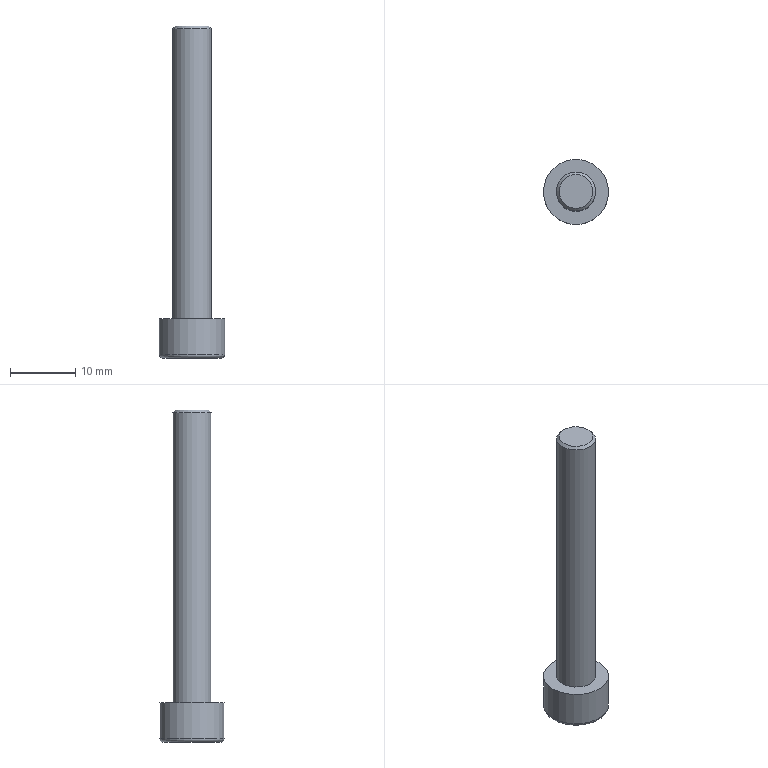Part | STEP file | 200 mesh_id134_x | 1 solid | 20 faces | box 10 x 10 x 51 mm | volume 1654 mm3 | plane 10 | cylinder 8 | torus 1 | cone 1 | commonest cylinder face diameters 0.4 x6 6 x1 10 x1
STEP:
#1=CARTESIAN_POINT('',(-16734.384,-3900.387,88.258));
#2=VERTEX_POINT('',#1);
#3=CARTESIAN_POINT('',(-16731.684,-3898.828,88.258));
#4=VERTEX_POINT('',#3);
#5=CARTESIAN_POINT('',(-16731.784,-3898.886,88.258));
#6=DIRECTION('',(0.866,0.5,0.));
#7=VECTOR('',#6,1.);
#8=LINE('',#5,#7);
#9=EDGE_CURVE('',#2,#4,#8,.T.);
#10=ORIENTED_EDGE('',*,*,#9,.T.);
#11=CARTESIAN_POINT('',(-16731.684,-3895.71,88.258));
#12=VERTEX_POINT('',#11);
#13=CARTESIAN_POINT('',(-16731.684,-3895.826,88.258));
#14=DIRECTION('',(0.,1.,0.));
#15=VECTOR('',#14,1.);
#16=LINE('',#13,#15);
#17=EDGE_CURVE('',#4,#12,#16,.T.);
#18=ORIENTED_EDGE('',*,*,#17,.T.);
#19=CARTESIAN_POINT('',(-16734.384,-3894.151,88.258));
#20=VERTEX_POINT('',#19);
#21=CARTESIAN_POINT('',(-16734.284,-3894.209,88.258));
#22=DIRECTION('',(-0.866,0.5,0.));
#23=VECTOR('',#22,1.);
#24=LINE('',#21,#23);
#25=EDGE_CURVE('',#12,#20,#24,.T.);
#26=ORIENTED_EDGE('',*,*,#25,.T.);
#27=CARTESIAN_POINT('',(-16737.084,-3895.71,88.258));
#28=VERTEX_POINT('',#27);
#29=CARTESIAN_POINT('',(-16736.984,-3895.653,88.258));
#30=DIRECTION('',(-0.866,-0.5,0.));
#31=VECTOR('',#30,1.);
#32=LINE('',#29,#31);
#33=EDGE_CURVE('',#20,#28,#32,.T.);
#34=ORIENTED_EDGE('',*,*,#33,.T.);
#35=CARTESIAN_POINT('',(-16737.084,-3898.828,88.258));
#36=VERTEX_POINT('',#35);
#37=CARTESIAN_POINT('',(-16737.084,-3898.713,88.258));
#38=DIRECTION('',(0.,-1.,0.));
#39=VECTOR('',#38,1.);
#40=LINE('',#37,#39);
#41=EDGE_CURVE('',#28,#36,#40,.T.);
#42=ORIENTED_EDGE('',*,*,#41,.T.);
#43=CARTESIAN_POINT('',(-16734.484,-3900.329,88.258));
#44=DIRECTION('',(0.866,-0.5,0.));
#45=VECTOR('',#44,1.);
#46=LINE('',#43,#45);
#47=EDGE_CURVE('',#36,#2,#46,.T.);
#48=ORIENTED_EDGE('',*,*,#47,.T.);
#49=EDGE_LOOP('',(#10,#18,#26,#34,#42,#48));
#50=FACE_BOUND('',#49,.T.);
#51=CARTESIAN_POINT('',(-16738.884,-3897.269,88.258));
#52=VERTEX_POINT('',#51);
#53=CARTESIAN_POINT('',(-16734.384,-3897.269,88.258));
#54=DIRECTION('',(0.,0.,-1.));
#55=DIRECTION('',(-1.,0.,0.));
#56=AXIS2_PLACEMENT_3D('',#53,#54,#55);
#57=CIRCLE('',#56,4.5);
#58=EDGE_CURVE('',#52,#52,#57,.T.);
#59=ORIENTED_EDGE('',*,*,#58,.T.);
#60=EDGE_LOOP('',(#59));
#61=FACE_BOUND('',#60,.T.);
#62=CARTESIAN_POINT('',(-16734.384,-3897.269,88.258));
#63=DIRECTION('',(0.,0.,-1.));
#64=DIRECTION('',(-1.,0.,0.));
#65=AXIS2_PLACEMENT_3D('',#62,#63,#64);
#66=PLANE('',#65);
#67=ADVANCED_FACE('',(#50,#61),#66,.T.);
#68=CARTESIAN_POINT('',(-16731.384,-3897.269,138.858));
#69=VERTEX_POINT('',#68);
#70=CARTESIAN_POINT('',(-16734.384,-3897.269,138.858));
#71=DIRECTION('',(0.,0.,-1.));
#72=DIRECTION('',(1.,0.,0.));
#73=AXIS2_PLACEMENT_3D('',#70,#71,#72);
#74=CIRCLE('',#73,3.);
#75=EDGE_CURVE('',#69,#69,#74,.T.);
#76=ORIENTED_EDGE('',*,*,#75,.T.);
#77=EDGE_LOOP('',(#76));
#78=FACE_BOUND('',#77,.T.);
#79=CARTESIAN_POINT('',(-16731.384,-3897.269,94.258));
#80=VERTEX_POINT('',#79);
#81=CARTESIAN_POINT('',(-16734.384,-3897.269,94.258));
#82=DIRECTION('',(0.,0.,-1.));
#83=DIRECTION('',(1.,0.,0.));
#84=AXIS2_PLACEMENT_3D('',#81,#82,#83);
#85=CIRCLE('',#84,3.);
#86=EDGE_CURVE('',#80,#80,#85,.T.);
#87=ORIENTED_EDGE('',*,*,#86,.F.);
#88=EDGE_LOOP('',(#87));
#89=FACE_BOUND('',#88,.T.);
#90=CARTESIAN_POINT('',(-16734.384,-3897.269,94.258));
#91=DIRECTION('',(0.,0.,1.));
#92=DIRECTION('',(1.,0.,0.));
#93=AXIS2_PLACEMENT_3D('',#90,#91,#92);
#94=CYLINDRICAL_SURFACE('',#93,3.);
#95=ADVANCED_FACE('',(#78,#89),#94,.T.);
#96=ORIENTED_EDGE('',*,*,#86,.T.);
#97=EDGE_LOOP('',(#96));
#98=FACE_BOUND('',#97,.T.);
#99=CARTESIAN_POINT('',(-16729.384,-3897.269,94.258));
#100=VERTEX_POINT('',#99);
#101=CARTESIAN_POINT('',(-16734.384,-3897.269,94.258));
#102=DIRECTION('',(0.,0.,-1.));
#103=DIRECTION('',(1.,0.,0.));
#104=AXIS2_PLACEMENT_3D('',#101,#102,#103);
#105=CIRCLE('',#104,5.);
#106=EDGE_CURVE('',#100,#100,#105,.T.);
#107=ORIENTED_EDGE('',*,*,#106,.F.);
#108=EDGE_LOOP('',(#107));
#109=FACE_BOUND('',#108,.T.);
#110=CARTESIAN_POINT('',(-16734.384,-3897.269,94.258));
#111=DIRECTION('',(0.,0.,1.));
#112=DIRECTION('',(1.,0.,0.));
#113=AXIS2_PLACEMENT_3D('',#110,#111,#112);
#114=PLANE('',#113);
#115=ADVANCED_FACE('',(#98,#109),#114,.T.);
#116=CARTESIAN_POINT('',(-16739.384,-3897.269,88.758));
#117=VERTEX_POINT('',#116);
#118=CARTESIAN_POINT('',(-16734.384,-3897.269,88.758));
#119=DIRECTION('',(0.,0.,1.));
#120=DIRECTION('',(-1.,0.,0.));
#121=AXIS2_PLACEMENT_3D('',#118,#119,#120);
#122=CIRCLE('',#121,5.);
#123=EDGE_CURVE('',#117,#117,#122,.T.);
#124=ORIENTED_EDGE('',*,*,#123,.T.);
#125=EDGE_LOOP('',(#124));
#126=FACE_BOUND('',#125,.T.);
#127=ORIENTED_EDGE('',*,*,#106,.T.);
#128=EDGE_LOOP('',(#127));
#129=FACE_BOUND('',#128,.T.);
#130=CARTESIAN_POINT('',(-16734.384,-3897.269,94.258));
#131=DIRECTION('',(0.,0.,-1.));
#132=DIRECTION('',(1.,0.,0.));
#133=AXIS2_PLACEMENT_3D('',#130,#131,#132);
#134=CYLINDRICAL_SURFACE('',#133,5.);
#135=ADVANCED_FACE('',(#126,#129),#134,.T.);
#136=ORIENTED_EDGE('',*,*,#58,.F.);
#137=EDGE_LOOP('',(#136));
#138=FACE_BOUND('',#137,.T.);
#139=ORIENTED_EDGE('',*,*,#123,.F.);
#140=EDGE_LOOP('',(#139));
#141=FACE_BOUND('',#140,.T.);
#142=CARTESIAN_POINT('',(-16734.384,-3897.269,88.758));
#143=DIRECTION('',(0.,0.,-1.));
#144=DIRECTION('',(-1.,0.,0.));
#145=AXIS2_PLACEMENT_3D('',#142,#143,#144);
#146=TOROIDAL_SURFACE('',#145,4.5,0.5);
#147=ADVANCED_FACE('',(#138,#141),#146,.T.);
#148=CARTESIAN_POINT('',(-16734.384,-3894.382,92.258));
#149=VERTEX_POINT('',#148);
#150=CARTESIAN_POINT('',(-16734.384,-3894.382,88.458));
#151=VERTEX_POINT('',#150);
#152=CARTESIAN_POINT('',(-16734.384,-3894.382,88.258));
#153=DIRECTION('',(0.,0.,-1.));
#154=VECTOR('',#153,1.);
#155=LINE('',#152,#154);
#156=EDGE_CURVE('',#149,#151,#155,.T.);
#157=ORIENTED_EDGE('',*,*,#156,.T.);
#158=CARTESIAN_POINT('',(-16731.884,-3895.826,88.458));
#159=VERTEX_POINT('',#158);
#160=CARTESIAN_POINT('',(-16731.884,-3895.826,88.458));
#161=DIRECTION('',(0.866,-0.5,0.));
#162=VECTOR('',#161,1.);
#163=LINE('',#160,#162);
#164=EDGE_CURVE('',#151,#159,#163,.T.);
#165=ORIENTED_EDGE('',*,*,#164,.T.);
#166=CARTESIAN_POINT('',(-16731.884,-3895.826,92.258));
#167=VERTEX_POINT('',#166);
#168=CARTESIAN_POINT('',(-16731.884,-3895.826,88.258));
#169=DIRECTION('',(0.,0.,-1.));
#170=VECTOR('',#169,1.);
#171=LINE('',#168,#170);
#172=EDGE_CURVE('',#167,#159,#171,.T.);
#173=ORIENTED_EDGE('',*,*,#172,.F.);
#174=CARTESIAN_POINT('',(-16731.884,-3895.826,92.258));
#175=DIRECTION('',(0.866,-0.5,0.));
#176=VECTOR('',#175,1.);
#177=LINE('',#174,#176);
#178=EDGE_CURVE('',#149,#167,#177,.T.);
#179=ORIENTED_EDGE('',*,*,#178,.F.);
#180=EDGE_LOOP('',(#157,#165,#173,#179));
#181=FACE_OUTER_BOUND('',#180,.T.);
#182=CARTESIAN_POINT('',(-16731.884,-3895.826,88.258));
#183=DIRECTION('',(0.5,0.866,0.));
#184=DIRECTION('',(-0.866,0.5,0.));
#185=AXIS2_PLACEMENT_3D('',#182,#183,#184);
#186=PLANE('',#185);
#187=ADVANCED_FACE('',(#181),#186,.F.);
#188=CARTESIAN_POINT('',(-16736.884,-3895.826,92.258));
#189=VERTEX_POINT('',#188);
#190=CARTESIAN_POINT('',(-16736.884,-3895.826,88.458));
#191=VERTEX_POINT('',#190);
#192=CARTESIAN_POINT('',(-16736.884,-3895.826,88.258));
#193=DIRECTION('',(0.,0.,-1.));
#194=VECTOR('',#193,1.);
#195=LINE('',#192,#194);
#196=EDGE_CURVE('',#189,#191,#195,.T.);
#197=ORIENTED_EDGE('',*,*,#196,.T.);
#198=CARTESIAN_POINT('',(-16734.384,-3894.382,88.458));
#199=DIRECTION('',(0.866,0.5,0.));
#200=VECTOR('',#199,1.);
#201=LINE('',#198,#200);
#202=EDGE_CURVE('',#191,#151,#201,.T.);
#203=ORIENTED_EDGE('',*,*,#202,.T.);
#204=ORIENTED_EDGE('',*,*,#156,.F.);
#205=CARTESIAN_POINT('',(-16734.384,-3894.382,92.258));
#206=DIRECTION('',(0.866,0.5,0.));
#207=VECTOR('',#206,1.);
#208=LINE('',#205,#207);
#209=EDGE_CURVE('',#189,#149,#208,.T.);
#210=ORIENTED_EDGE('',*,*,#209,.F.);
#211=EDGE_LOOP('',(#197,#203,#204,#210));
#212=FACE_OUTER_BOUND('',#211,.T.);
#213=CARTESIAN_POINT('',(-16734.384,-3894.382,88.258));
#214=DIRECTION('',(-0.5,0.866,0.));
#215=DIRECTION('',(-0.866,-0.5,0.));
#216=AXIS2_PLACEMENT_3D('',#213,#214,#215);
#217=PLANE('',#216);
#218=ADVANCED_FACE('',(#212),#217,.F.);
#219=CARTESIAN_POINT('',(-16736.884,-3898.713,92.258));
#220=VERTEX_POINT('',#219);
#221=CARTESIAN_POINT('',(-16736.884,-3898.713,88.458));
#222=VERTEX_POINT('',#221);
#223=CARTESIAN_POINT('',(-16736.884,-3898.713,88.258));
#224=DIRECTION('',(0.,0.,-1.));
#225=VECTOR('',#224,1.);
#226=LINE('',#223,#225);
#227=EDGE_CURVE('',#220,#222,#226,.T.);
#228=ORIENTED_EDGE('',*,*,#227,.T.);
#229=CARTESIAN_POINT('',(-16736.884,-3895.826,88.458));
#230=DIRECTION('',(0.,1.,0.));
#231=VECTOR('',#230,1.);
#232=LINE('',#229,#231);
#233=EDGE_CURVE('',#222,#191,#232,.T.);
#234=ORIENTED_EDGE('',*,*,#233,.T.);
#235=ORIENTED_EDGE('',*,*,#196,.F.);
#236=CARTESIAN_POINT('',(-16736.884,-3895.826,92.258));
#237=DIRECTION('',(0.,1.,0.));
#238=VECTOR('',#237,1.);
#239=LINE('',#236,#238);
#240=EDGE_CURVE('',#220,#189,#239,.T.);
#241=ORIENTED_EDGE('',*,*,#240,.F.);
#242=EDGE_LOOP('',(#228,#234,#235,#241));
#243=FACE_OUTER_BOUND('',#242,.T.);
#244=CARTESIAN_POINT('',(-16736.884,-3895.826,88.258));
#245=DIRECTION('',(-1.,0.,0.));
#246=DIRECTION('',(0.,0.,1.));
#247=AXIS2_PLACEMENT_3D('',#244,#245,#246);
#248=PLANE('',#247);
#249=ADVANCED_FACE('',(#243),#248,.F.);
#250=CARTESIAN_POINT('',(-16734.384,-3900.156,92.258));
#251=VERTEX_POINT('',#250);
#252=CARTESIAN_POINT('',(-16734.384,-3900.156,88.458));
#253=VERTEX_POINT('',#252);
#254=CARTESIAN_POINT('',(-16734.384,-3900.156,88.258));
#255=DIRECTION('',(0.,0.,-1.));
#256=VECTOR('',#255,1.);
#257=LINE('',#254,#256);
#258=EDGE_CURVE('',#251,#253,#257,.T.);
#259=ORIENTED_EDGE('',*,*,#258,.T.);
#260=CARTESIAN_POINT('',(-16736.884,-3898.713,88.458));
#261=DIRECTION('',(-0.866,0.5,0.));
#262=VECTOR('',#261,1.);
#263=LINE('',#260,#262);
#264=EDGE_CURVE('',#253,#222,#263,.T.);
#265=ORIENTED_EDGE('',*,*,#264,.T.);
#266=ORIENTED_EDGE('',*,*,#227,.F.);
#267=CARTESIAN_POINT('',(-16736.884,-3898.713,92.258));
#268=DIRECTION('',(-0.866,0.5,0.));
#269=VECTOR('',#268,1.);
#270=LINE('',#267,#269);
#271=EDGE_CURVE('',#251,#220,#270,.T.);
#272=ORIENTED_EDGE('',*,*,#271,.F.);
#273=EDGE_LOOP('',(#259,#265,#266,#272));
#274=FACE_OUTER_BOUND('',#273,.T.);
#275=CARTESIAN_POINT('',(-16736.884,-3898.713,88.258));
#276=DIRECTION('',(-0.5,-0.866,0.));
#277=DIRECTION('',(0.866,-0.5,0.));
#278=AXIS2_PLACEMENT_3D('',#275,#276,#277);
#279=PLANE('',#278);
#280=ADVANCED_FACE('',(#274),#279,.F.);
#281=CARTESIAN_POINT('',(-16731.884,-3898.713,92.258));
#282=VERTEX_POINT('',#281);
#283=CARTESIAN_POINT('',(-16731.884,-3898.713,88.458));
#284=VERTEX_POINT('',#283);
#285=CARTESIAN_POINT('',(-16731.884,-3898.713,88.258));
#286=DIRECTION('',(0.,0.,-1.));
#287=VECTOR('',#286,1.);
#288=LINE('',#285,#287);
#289=EDGE_CURVE('',#282,#284,#288,.T.);
#290=ORIENTED_EDGE('',*,*,#289,.T.);
#291=CARTESIAN_POINT('',(-16734.384,-3900.156,88.458));
#292=DIRECTION('',(-0.866,-0.5,0.));
#293=VECTOR('',#292,1.);
#294=LINE('',#291,#293);
#295=EDGE_CURVE('',#284,#253,#294,.T.);
#296=ORIENTED_EDGE('',*,*,#295,.T.);
#297=ORIENTED_EDGE('',*,*,#258,.F.);
#298=CARTESIAN_POINT('',(-16734.384,-3900.156,92.258));
#299=DIRECTION('',(-0.866,-0.5,0.));
#300=VECTOR('',#299,1.);
#301=LINE('',#298,#300);
#302=EDGE_CURVE('',#282,#251,#301,.T.);
#303=ORIENTED_EDGE('',*,*,#302,.F.);
#304=EDGE_LOOP('',(#290,#296,#297,#303));
#305=FACE_OUTER_BOUND('',#304,.T.);
#306=CARTESIAN_POINT('',(-16734.384,-3900.156,88.258));
#307=DIRECTION('',(0.5,-0.866,0.));
#308=DIRECTION('',(0.866,0.5,0.));
#309=AXIS2_PLACEMENT_3D('',#306,#307,#308);
#310=PLANE('',#309);
#311=ADVANCED_FACE('',(#305),#310,.F.);
#312=ORIENTED_EDGE('',*,*,#172,.T.);
#313=CARTESIAN_POINT('',(-16731.884,-3898.713,88.458));
#314=DIRECTION('',(0.,-1.,0.));
#315=VECTOR('',#314,1.);
#316=LINE('',#313,#315);
#317=EDGE_CURVE('',#159,#284,#316,.T.);
#318=ORIENTED_EDGE('',*,*,#317,.T.);
#319=ORIENTED_EDGE('',*,*,#289,.F.);
#320=CARTESIAN_POINT('',(-16731.884,-3898.713,92.258));
#321=DIRECTION('',(0.,-1.,0.));
#322=VECTOR('',#321,1.);
#323=LINE('',#320,#322);
#324=EDGE_CURVE('',#167,#282,#323,.T.);
#325=ORIENTED_EDGE('',*,*,#324,.F.);
#326=EDGE_LOOP('',(#312,#318,#319,#325));
#327=FACE_OUTER_BOUND('',#326,.T.);
#328=CARTESIAN_POINT('',(-16731.884,-3898.713,88.258));
#329=DIRECTION('',(1.,0.,0.));
#330=DIRECTION('',(0.,0.,-1.));
#331=AXIS2_PLACEMENT_3D('',#328,#329,#330);
#332=PLANE('',#331);
#333=ADVANCED_FACE('',(#327),#332,.F.);
#334=ORIENTED_EDGE('',*,*,#178,.T.);
#335=ORIENTED_EDGE('',*,*,#324,.T.);
#336=ORIENTED_EDGE('',*,*,#302,.T.);
#337=ORIENTED_EDGE('',*,*,#271,.T.);
#338=ORIENTED_EDGE('',*,*,#240,.T.);
#339=ORIENTED_EDGE('',*,*,#209,.T.);
#340=EDGE_LOOP('',(#334,#335,#336,#337,#338,#339));
#341=FACE_OUTER_BOUND('',#340,.T.);
#342=CARTESIAN_POINT('',(116.,246.,92.258));
#343=DIRECTION('',(0.,0.,1.));
#344=DIRECTION('',(1.,0.,0.));
#345=AXIS2_PLACEMENT_3D('',#342,#343,#344);
#346=PLANE('',#345);
#347=ADVANCED_FACE('',(#341),#346,.F.);
#348=CARTESIAN_POINT('',(-16737.084,-3895.71,88.458));
#349=DIRECTION('',(0.5,0.866,0.));
#350=DIRECTION('',(0.866,-0.5,0.));
#351=AXIS2_PLACEMENT_3D('',#348,#349,#350);
#352=ELLIPSE('',#351,0.2309,0.2);
#353=EDGE_CURVE('',#191,#28,#352,.T.);
#354=ORIENTED_EDGE('',*,*,#353,.F.);
#355=ORIENTED_EDGE('',*,*,#233,.F.);
#356=CARTESIAN_POINT('',(-16737.084,-3898.828,88.458));
#357=DIRECTION('',(0.5,-0.866,0.));
#358=DIRECTION('',(0.866,0.5,0.));
#359=AXIS2_PLACEMENT_3D('',#356,#357,#358);
#360=ELLIPSE('',#359,0.2309,0.2);
#361=EDGE_CURVE('',#36,#222,#360,.T.);
#362=ORIENTED_EDGE('',*,*,#361,.F.);
#363=ORIENTED_EDGE('',*,*,#41,.F.);
#364=EDGE_LOOP('',(#354,#355,#362,#363));
#365=FACE_OUTER_BOUND('',#364,.T.);
#366=CARTESIAN_POINT('',(-16737.084,-3897.269,88.458));
#367=DIRECTION('',(0.,1.,0.));
#368=DIRECTION('',(0.,0.,1.));
#369=AXIS2_PLACEMENT_3D('',#366,#367,#368);
#370=CYLINDRICAL_SURFACE('',#369,0.2);
#371=ADVANCED_FACE('',(#365),#370,.T.);
#372=ORIENTED_EDGE('',*,*,#361,.T.);
#373=ORIENTED_EDGE('',*,*,#264,.F.);
#374=CARTESIAN_POINT('',(-16734.384,-3900.387,88.458));
#375=DIRECTION('',(1.,0.,0.));
#376=DIRECTION('',(0.,1.,0.));
#377=AXIS2_PLACEMENT_3D('',#374,#375,#376);
#378=ELLIPSE('',#377,0.2309,0.2);
#379=EDGE_CURVE('',#2,#253,#378,.T.);
#380=ORIENTED_EDGE('',*,*,#379,.F.);
#381=ORIENTED_EDGE('',*,*,#47,.F.);
#382=EDGE_LOOP('',(#372,#373,#380,#381));
#383=FACE_OUTER_BOUND('',#382,.T.);
#384=CARTESIAN_POINT('',(-16735.734,-3899.607,88.458));
#385=DIRECTION('',(-0.866,0.5,0.));
#386=DIRECTION('',(-0.5,-0.866,0.));
#387=AXIS2_PLACEMENT_3D('',#384,#385,#386);
#388=CYLINDRICAL_SURFACE('',#387,0.2);
#389=ADVANCED_FACE('',(#383),#388,.T.);
#390=ORIENTED_EDGE('',*,*,#353,.T.);
#391=ORIENTED_EDGE('',*,*,#33,.F.);
#392=CARTESIAN_POINT('',(-16734.384,-3894.151,88.458));
#393=DIRECTION('',(1.,0.,0.));
#394=DIRECTION('',(0.,-1.,0.));
#395=AXIS2_PLACEMENT_3D('',#392,#393,#394);
#396=ELLIPSE('',#395,0.2309,0.2);
#397=EDGE_CURVE('',#151,#20,#396,.T.);
#398=ORIENTED_EDGE('',*,*,#397,.F.);
#399=ORIENTED_EDGE('',*,*,#202,.F.);
#400=EDGE_LOOP('',(#390,#391,#398,#399));
#401=FACE_OUTER_BOUND('',#400,.T.);
#402=CARTESIAN_POINT('',(-16735.734,-3894.931,88.458));
#403=DIRECTION('',(0.866,0.5,0.));
#404=DIRECTION('',(-0.5,0.866,0.));
#405=AXIS2_PLACEMENT_3D('',#402,#403,#404);
#406=CYLINDRICAL_SURFACE('',#405,0.2);
#407=ADVANCED_FACE('',(#401),#406,.T.);
#408=ORIENTED_EDGE('',*,*,#379,.T.);
#409=ORIENTED_EDGE('',*,*,#295,.F.);
#410=CARTESIAN_POINT('',(-16731.684,-3898.828,88.458));
#411=DIRECTION('',(0.5,0.866,0.));
#412=DIRECTION('',(0.866,-0.5,0.));
#413=AXIS2_PLACEMENT_3D('',#410,#411,#412);
#414=ELLIPSE('',#413,0.2309,0.2);
#415=EDGE_CURVE('',#4,#284,#414,.T.);
#416=ORIENTED_EDGE('',*,*,#415,.F.);
#417=ORIENTED_EDGE('',*,*,#9,.F.);
#418=EDGE_LOOP('',(#408,#409,#416,#417));
#419=FACE_OUTER_BOUND('',#418,.T.);
#420=CARTESIAN_POINT('',(-16733.034,-3899.607,88.458));
#421=DIRECTION('',(-0.866,-0.5,0.));
#422=DIRECTION('',(0.5,-0.866,0.));
#423=AXIS2_PLACEMENT_3D('',#420,#421,#422);
#424=CYLINDRICAL_SURFACE('',#423,0.2);
#425=ADVANCED_FACE('',(#419),#424,.T.);
#426=ORIENTED_EDGE('',*,*,#397,.T.);
#427=ORIENTED_EDGE('',*,*,#25,.F.);
#428=CARTESIAN_POINT('',(-16731.684,-3895.71,88.458));
#429=DIRECTION('',(0.5,-0.866,0.));
#430=DIRECTION('',(-0.866,-0.5,0.));
#431=AXIS2_PLACEMENT_3D('',#428,#429,#430);
#432=ELLIPSE('',#431,0.2309,0.2);
#433=EDGE_CURVE('',#159,#12,#432,.T.);
#434=ORIENTED_EDGE('',*,*,#433,.F.);
#435=ORIENTED_EDGE('',*,*,#164,.F.);
#436=EDGE_LOOP('',(#426,#427,#434,#435));
#437=FACE_OUTER_BOUND('',#436,.T.);
#438=CARTESIAN_POINT('',(-16733.034,-3894.931,88.458));
#439=DIRECTION('',(0.866,-0.5,0.));
#440=DIRECTION('',(0.5,0.866,0.));
#441=AXIS2_PLACEMENT_3D('',#438,#439,#440);
#442=CYLINDRICAL_SURFACE('',#441,0.2);
#443=ADVANCED_FACE('',(#437),#442,.T.);
#444=ORIENTED_EDGE('',*,*,#415,.T.);
#445=ORIENTED_EDGE('',*,*,#317,.F.);
#446=ORIENTED_EDGE('',*,*,#433,.T.);
#447=ORIENTED_EDGE('',*,*,#17,.F.);
#448=EDGE_LOOP('',(#444,#445,#446,#447));
#449=FACE_OUTER_BOUND('',#448,.T.);
#450=CARTESIAN_POINT('',(-16731.684,-3897.269,88.458));
#451=DIRECTION('',(0.,-1.,0.));
#452=DIRECTION('',(0.,0.,-1.));
#453=AXIS2_PLACEMENT_3D('',#450,#451,#452);
#454=CYLINDRICAL_SURFACE('',#453,0.2);
#455=ADVANCED_FACE('',(#449),#454,.T.);
#456=CARTESIAN_POINT('',(-16731.784,-3897.269,139.258));
#457=VERTEX_POINT('',#456);
#458=CARTESIAN_POINT('',(-16734.384,-3897.269,139.258));
#459=DIRECTION('',(0.,0.,1.));
#460=DIRECTION('',(1.,0.,0.));
#461=AXIS2_PLACEMENT_3D('',#458,#459,#460);
#462=CIRCLE('',#461,2.6);
#463=EDGE_CURVE('',#457,#457,#462,.T.);
#464=ORIENTED_EDGE('',*,*,#463,.T.);
#465=EDGE_LOOP('',(#464));
#466=FACE_OUTER_BOUND('',#465,.T.);
#467=CARTESIAN_POINT('',(-16734.384,-3897.269,139.258));
#468=DIRECTION('',(0.,0.,1.));
#469=DIRECTION('',(1.,0.,0.));
#470=AXIS2_PLACEMENT_3D('',#467,#468,#469);
#471=PLANE('',#470);
#472=ADVANCED_FACE('',(#466),#471,.T.);
#473=ORIENTED_EDGE('',*,*,#75,.F.);
#474=EDGE_LOOP('',(#473));
#475=FACE_BOUND('',#474,.T.);
#476=ORIENTED_EDGE('',*,*,#463,.F.);
#477=EDGE_LOOP('',(#476));
#478=FACE_BOUND('',#477,.T.);
#479=CARTESIAN_POINT('',(-16734.384,-3897.269,139.258));
#480=DIRECTION('',(0.,0.,-1.));
#481=DIRECTION('',(-1.,0.,0.));
#482=AXIS2_PLACEMENT_3D('',#479,#480,#481);
#483=CONICAL_SURFACE('',#482,2.6,45.);
#484=ADVANCED_FACE('',(#475,#478),#483,.T.);
#485=CLOSED_SHELL('',(#67,#95,#115,#135,#147,#187,#218,#249,#280,#311,#333,#347,#371,#389,#407,#425,#443,#455,#472,#484));
#486=MANIFOLD_SOLID_BREP('',#485);
#487=(LENGTH_UNIT()NAMED_UNIT(*)SI_UNIT(.MILLI.,.METRE.));
#488=UNCERTAINTY_MEASURE_WITH_UNIT(LENGTH_MEASURE(0.00002),#487,'','');
#489=(NAMED_UNIT(*)PLANE_ANGLE_UNIT()SI_UNIT($,.RADIAN.));
#490=PLANE_ANGLE_MEASURE_WITH_UNIT(PLANE_ANGLE_MEASURE(0.01745),#489);
#491=DIMENSIONAL_EXPONENTS(0.,0.,0.,0.,0.,0.,0.);
#492=(CONVERSION_BASED_UNIT('DEGREE',#490)NAMED_UNIT(#491)PLANE_ANGLE_UNIT());
#493=(NAMED_UNIT(*)SI_UNIT($,.STERADIAN.)SOLID_ANGLE_UNIT());
#494=(GEOMETRIC_REPRESENTATION_CONTEXT(3)GLOBAL_UNCERTAINTY_ASSIGNED_CONTEXT((#488))GLOBAL_UNIT_ASSIGNED_CONTEXT((#487,#492,#493))REPRESENTATION_CONTEXT('',''));
#495=ADVANCED_BREP_SHAPE_REPRESENTATION('',(#486),#494);